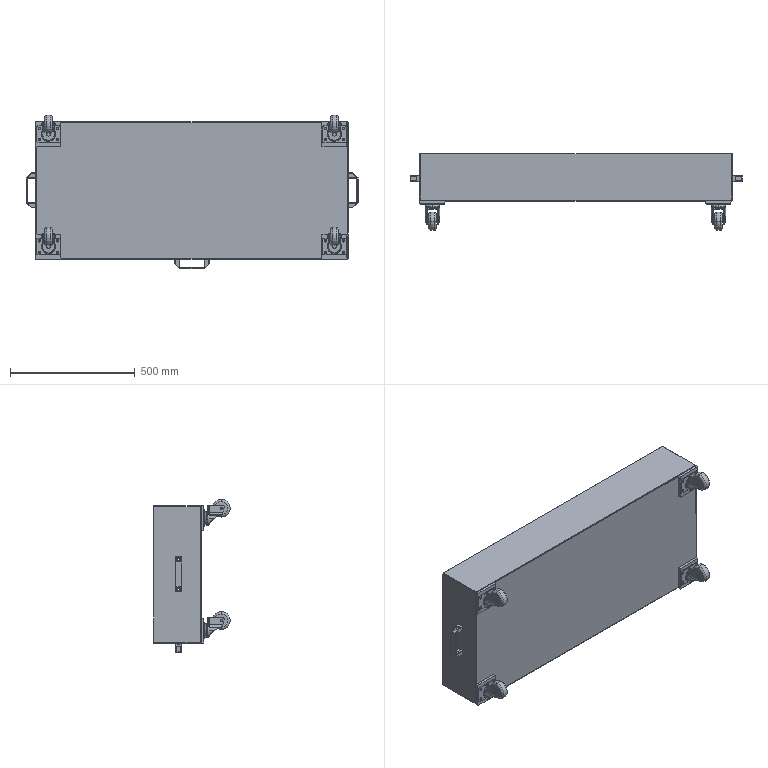Part | SolidWorks | features ReferencePattern 3, LocalLPattern 1 | 24 solids | 714 faces | box 1330 x 308 x 617 mm | volume 5317386 mm3 | cylinder 370 | plane 232 | torus 56 | spline 44 | sphere 12 | commonest cylinder face diameters 9 x76 2 x66 4 x32 6.8 x32 8 x24 10 x24